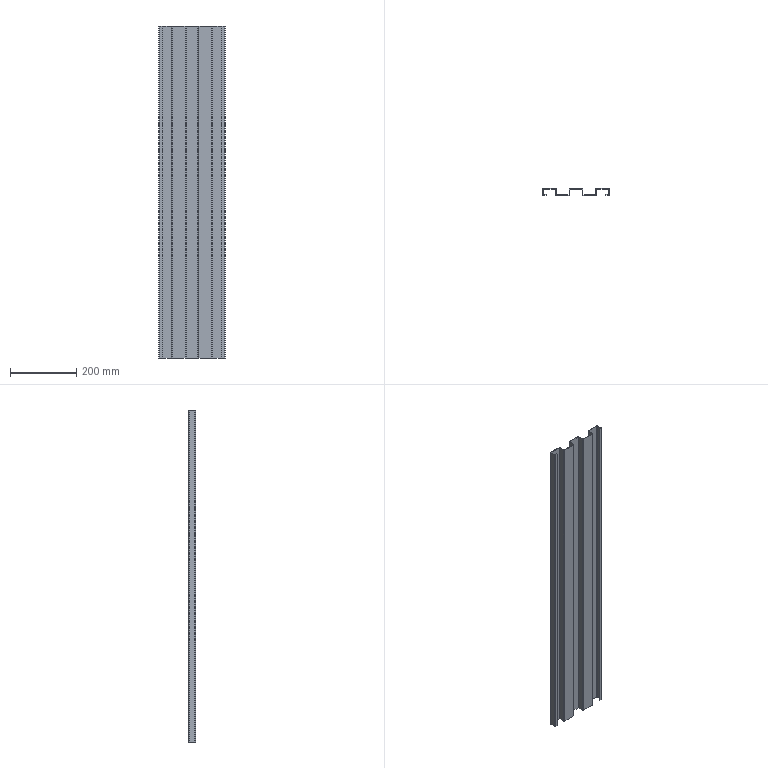Part | SolidWorks | features BaseBody 1 | 1 solid | 102 faces | box 200 x 21.2 x 1000 mm | volume 392351 mm3 | plane 78 | cylinder 24 | commonest cylinder face diameters 2 x12 4.4 x12